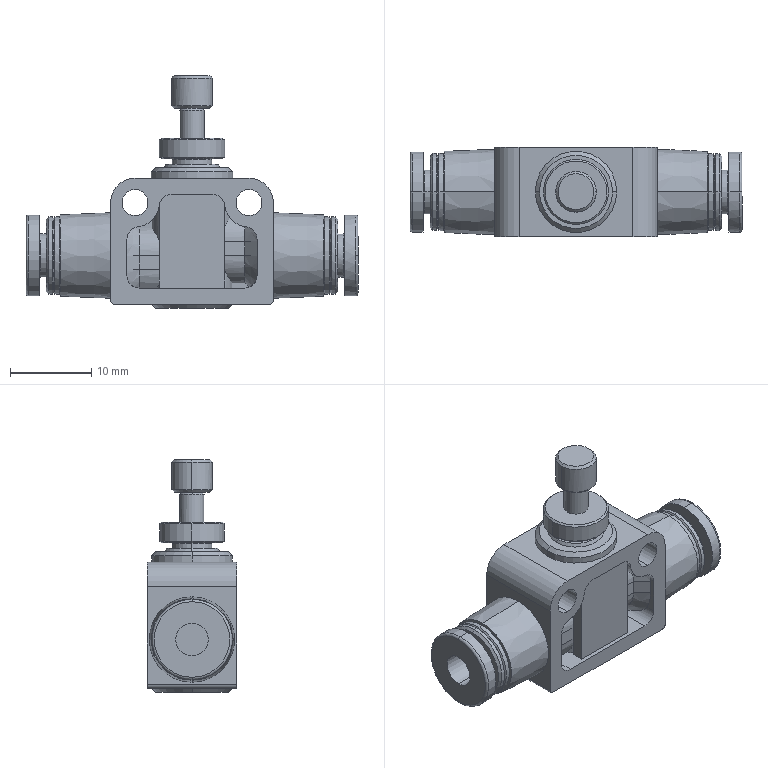Part | SolidWorks | features BaseBody 1 | 1 solid | 186 faces | box 40.8 x 11 x 28.611 mm | volume 4329 mm3 | cylinder 72 | cone 54 | plane 50 | torus 10 | commonest cylinder face diameters 3 x15 7 x8 9.5 x8 10 x7 3.2 x6 5.4 x6